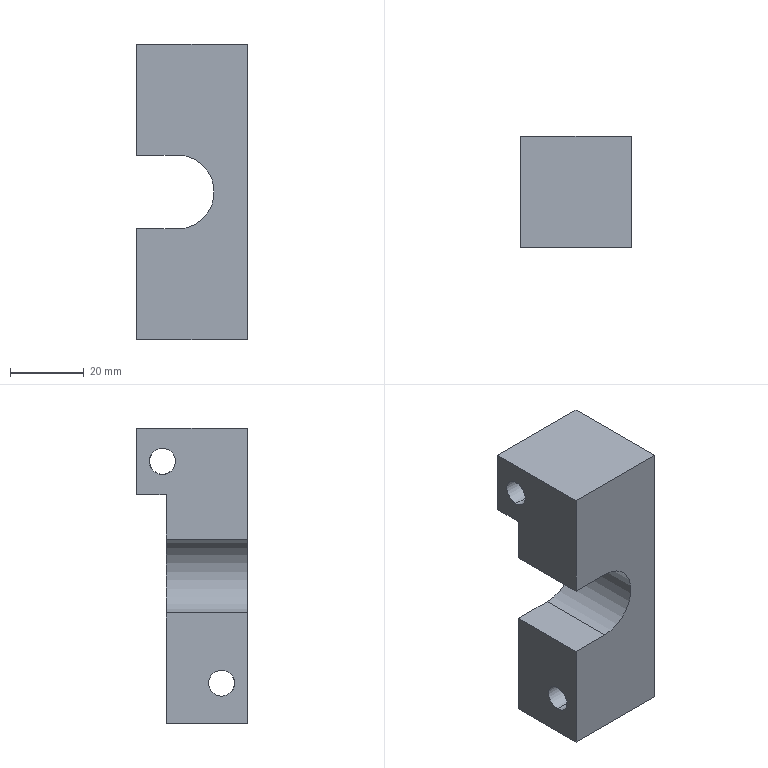Part | STEP file | OP10-127_cylinder base M6 | 1 solid | 38 faces | box 30 x 30 x 80 mm | volume 45481 mm3 | cylinder 13 | plane 13 | cone 12 | commonest cylinder face diameters 4.2 x4 7 x4 11 x4 20 x1